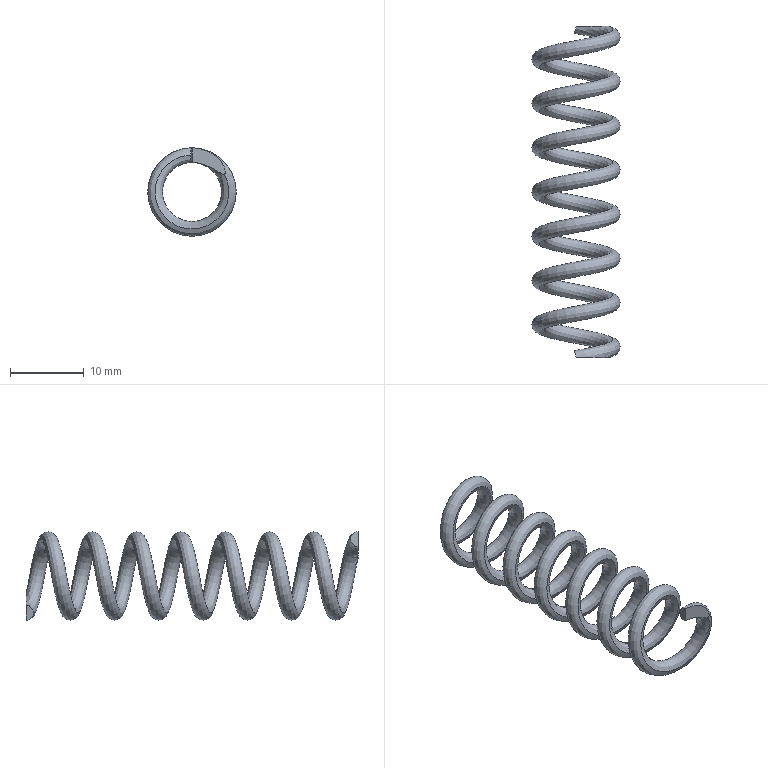Part | SolidWorks | features Helix 2, ICE 2, Sweep 2 | 1 solid | 6 faces | box 12 x 45 x 12 mm | volume 746.282 mm3 | plane 4 | spline 2